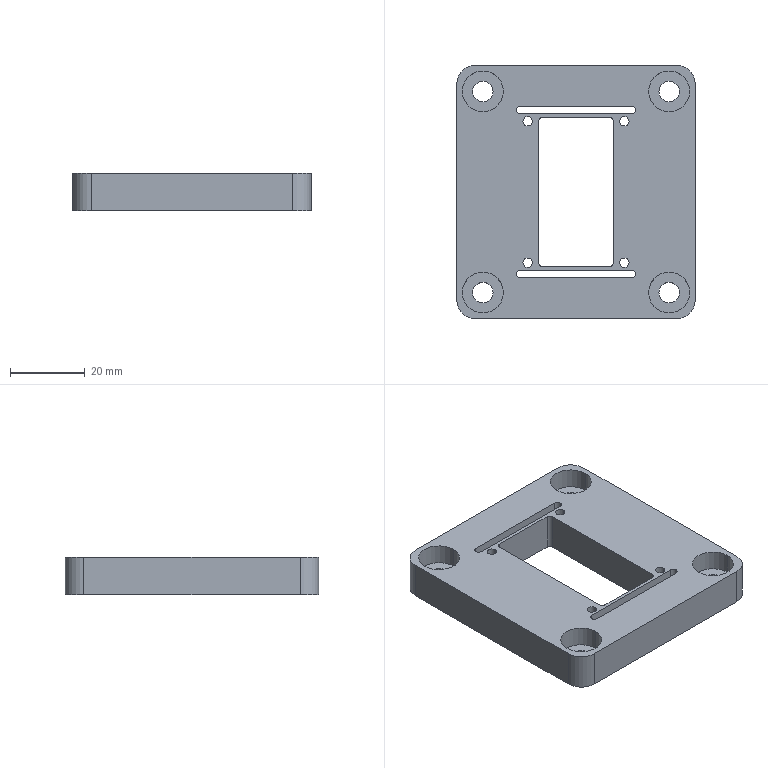Part | STEP file | MJ45 standard foot | 1 solid | 56 faces | box 64 x 68 x 10 mm | volume 31336 mm3 | cylinder 38 | plane 18 | commonest cylinder face diameters 2 x10 2.5 x8 5.5 x8 11 x8 10 x4